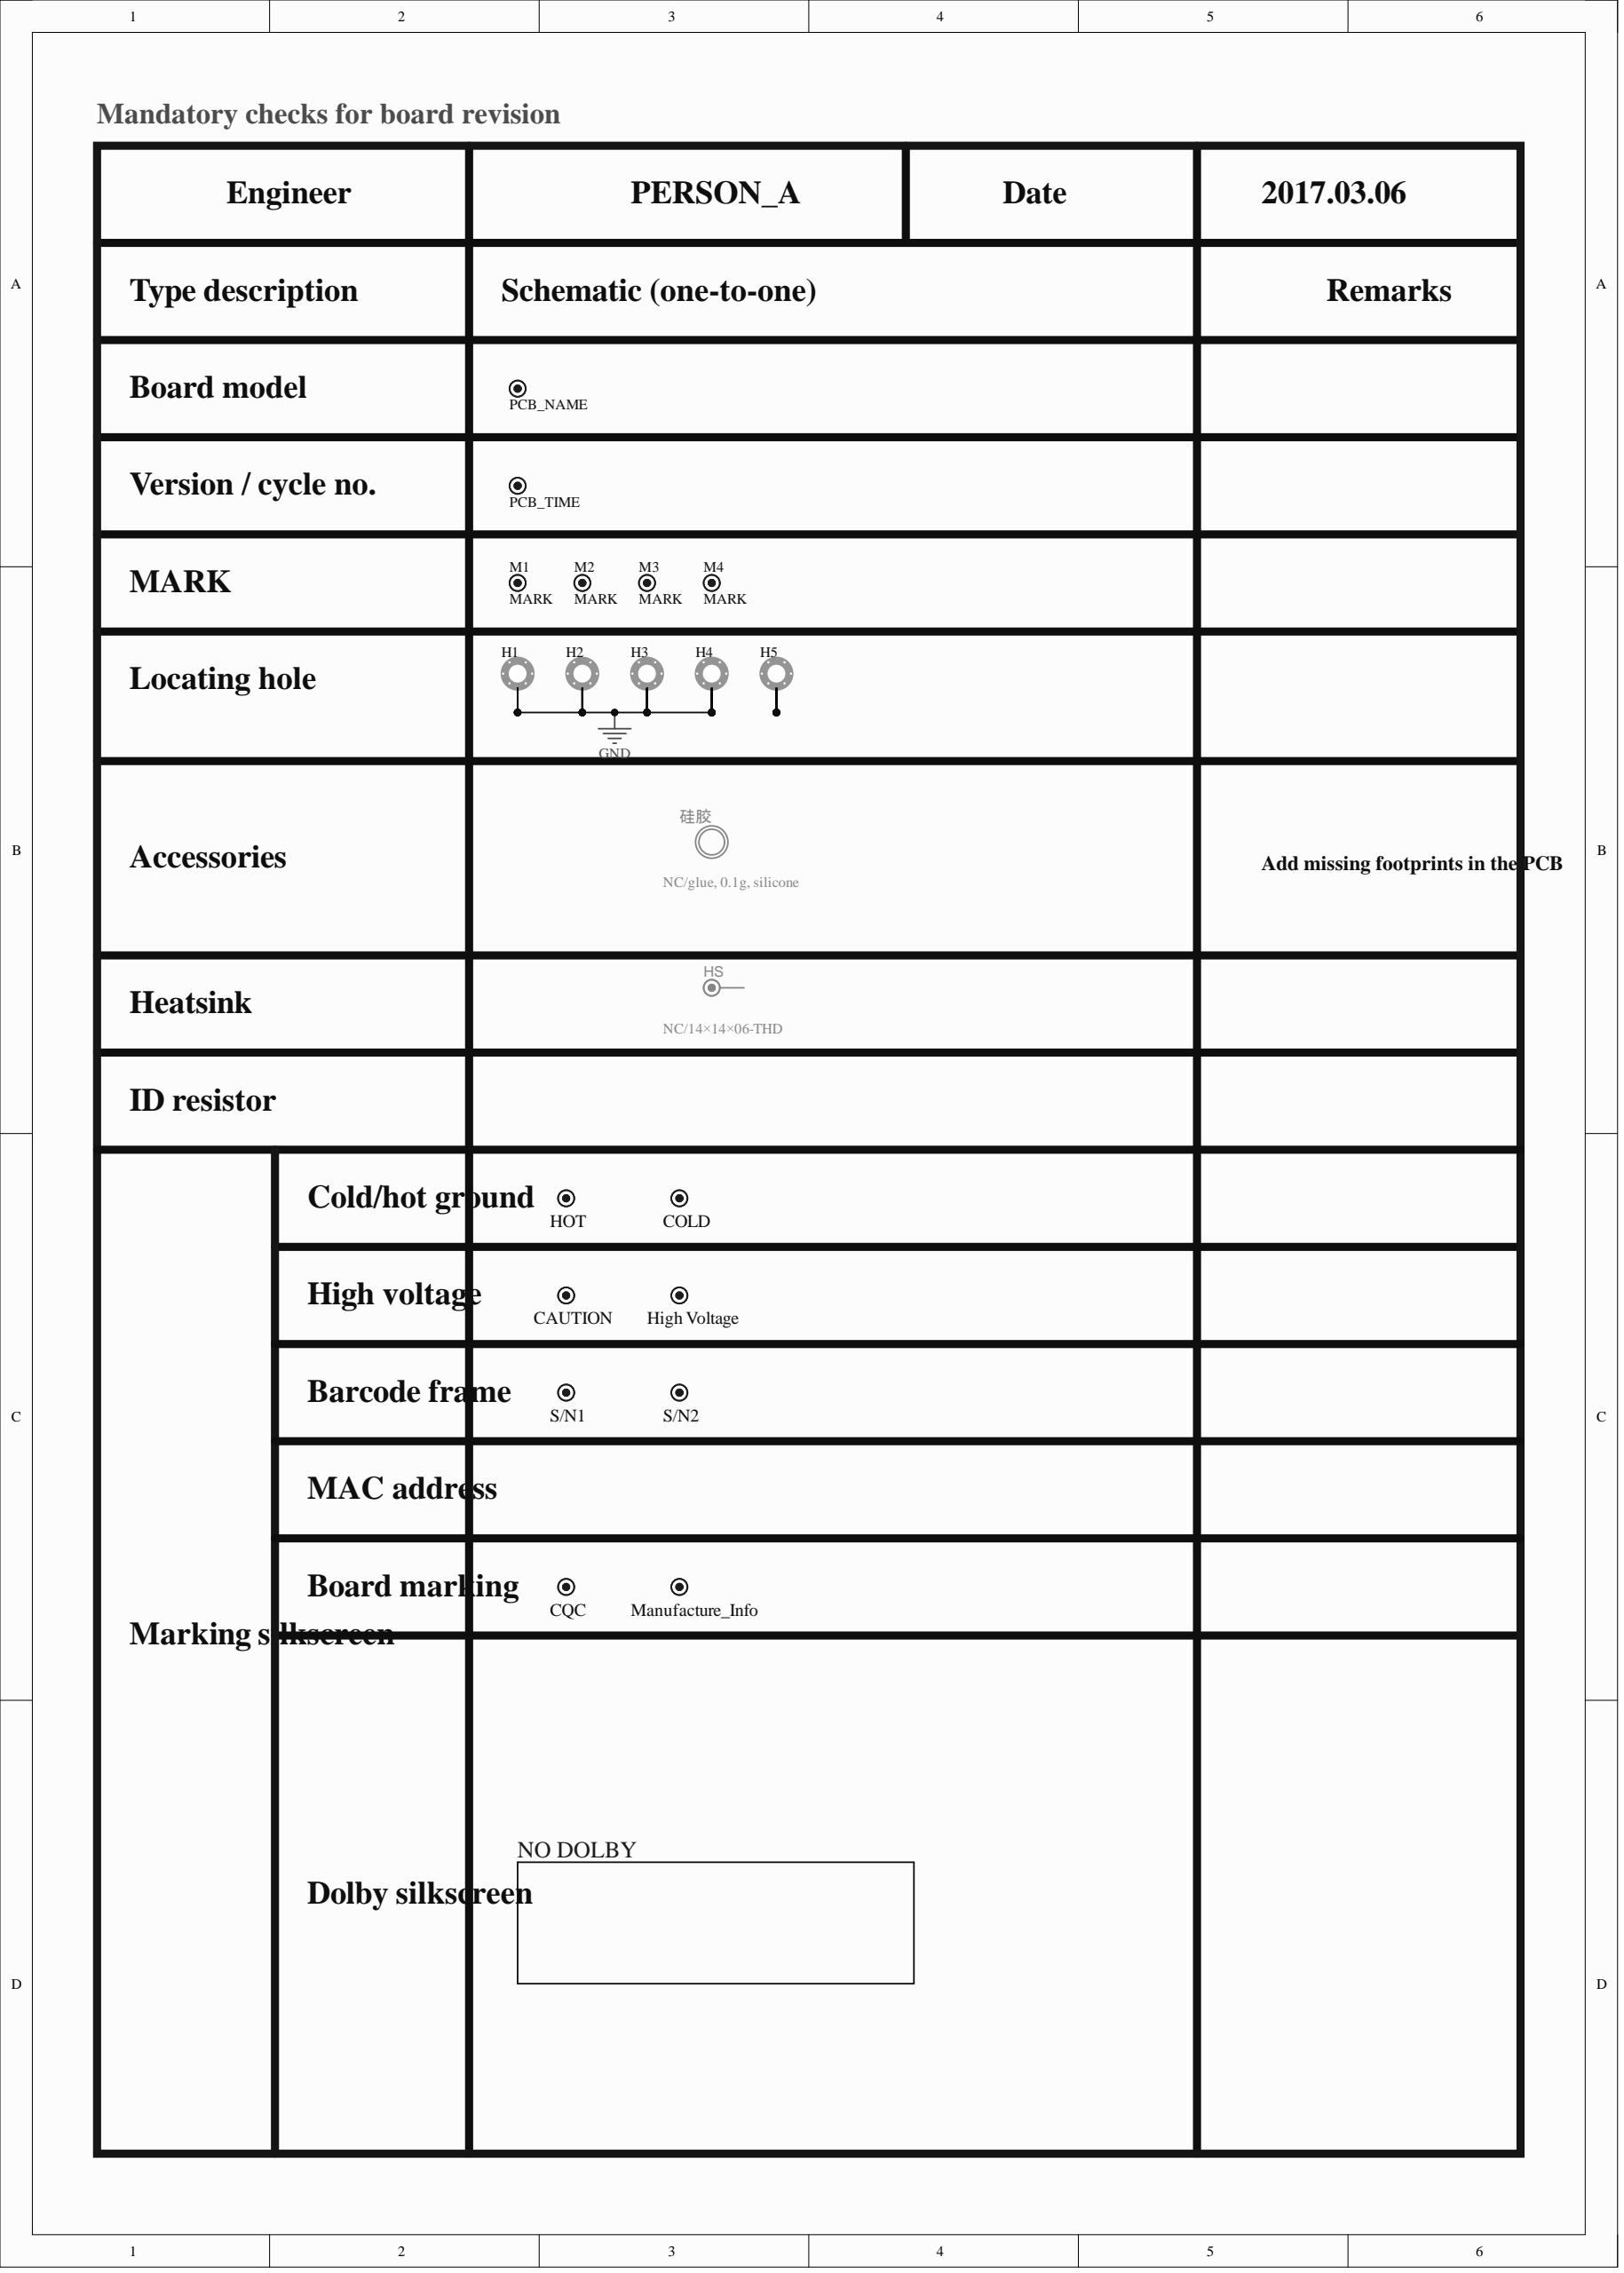Circuit board | Altium Designer | 709 parts | 378 nets | one sheet of the schematic
Parts on this sheet (reference | value | footprint):
CAUTION | CAUTION | CAUTION
COLD | COLD | COLD
CQC | CQC | CQC
H1 | Location hole | ASSE3.5C-3
H2 | Location hole | ASSE3.5C-3
H3 | Location hole | ASSE4.0C-4
H4 | Location hole | ASSE5.0C-4
H5 | Location hole | ASSE3.5C-3
HOT | HOT | HOT
HS | NC/14×14×06-THD | HS-S
M1 | MARK | MARK
M2 | MARK | MARK
M3 | MARK | MARK
M4 | MARK | MARK
Manufacture_Info | Manufacture_Info | Manufacture_Info
S/N1 | Barcode | Barcode
S/N2 | Barcode | Barcode
硅胶 | NC/glue, 0.1g, silicone | Heat-Shrinkable Tube
Nets of these parts (net: part-pin ...):
NetH5_0: H5-0 H5-1 H5-2 H5-3 H5-4 H5-5 H5-6
GND: H1-0 H1-1 H1-2 H1-3 H1-4 H1-5 H1-6 H2-0 H2-1 H2-2 H2-3 H2-4 H2-5 H2-6 H3-0 H3-1 H3-2 H3-3 H3-4 H3-5 H3-6 H4-0 H4-1 H4-2 H4-3 H4-4 H4-5 H4-6